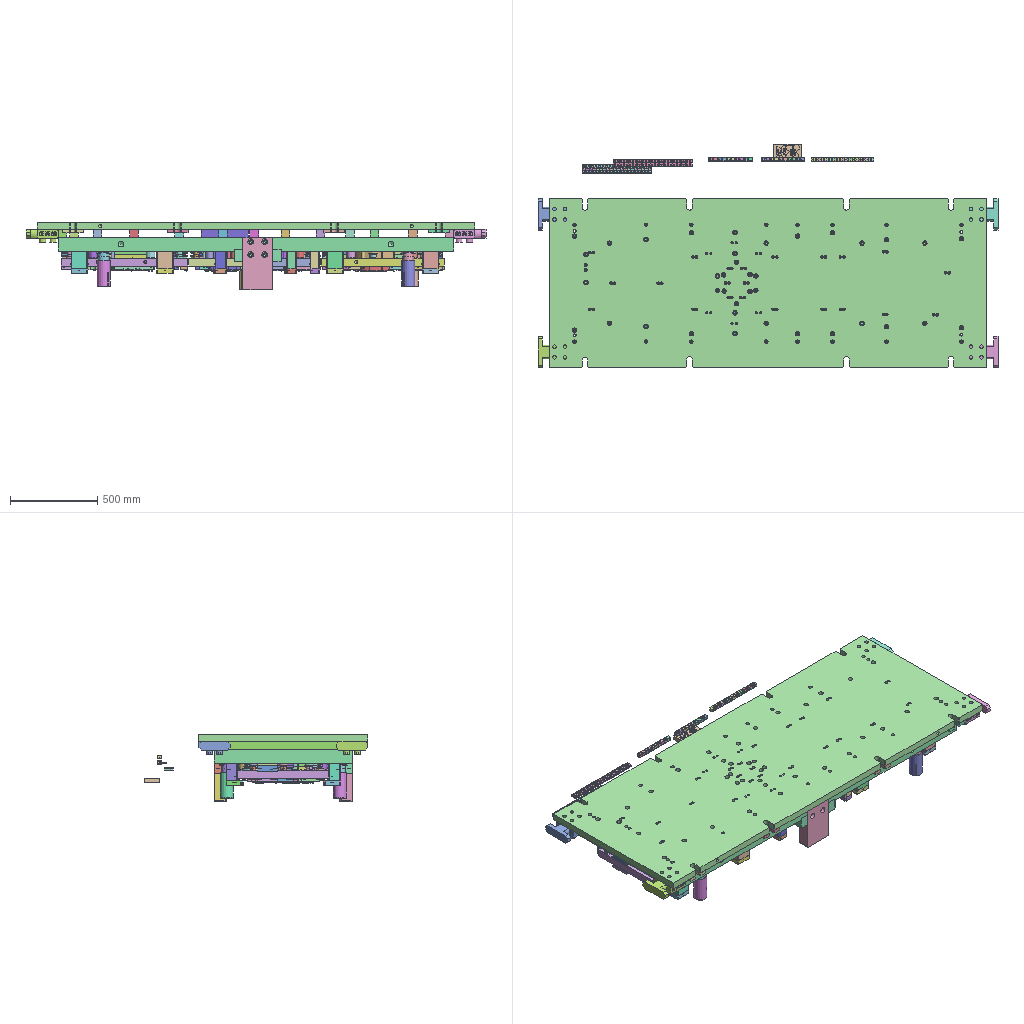Assembly | STEP file | 803 different items | 803 placed | box 2640 x 1282 x 385 mm
Parts list (item | name | quantity | parent item | size | volume), first 255 of 803 items:
1 | 1_id3214_x_t | x1 | in gslz 2016.10.28-10_x_t | 21 x 21 x 81 mm | 13603 mm3
2 | 1_id3210_x_t | x1 | in gslz 2016.10.28-10_x_t | 21 x 21 x 81 mm | 13603 mm3
3 | 1_id3206_x_t | x1 | in gslz 2016.10.28-10_x_t | 21 x 21 x 81 mm | 13603 mm3
4 | 1_id3202_x_t | x1 | in gslz 2016.10.28-10_x_t | 21 x 21 x 81 mm | 13603 mm3
5 | gslz 2016.10.28-10_id3198_x_t | x1 | in gslz 2016.10.28-10_x_t | 101.187 x 62.226 x 90 mm | 237811 mm3
6 | gslz 2016.10.28-10_id3194_x_t | x1 | in gslz 2016.10.28-10_x_t | 101.187 x 66.608 x 90 mm | 278822 mm3
7 | gslz 2016.10.28-10_id3190_x_t | x1 | in gslz 2016.10.28-10_x_t | 51.195 x 103.6 x 90 mm | 199398 mm3
8 | 107_id3186_x_t | x1 | in gslz 2016.10.28-10_x_t | 260 x 110 x 20 mm | 549192 mm3
9 | 105_id3182_x_t | x1 | in gslz 2016.10.28-10_x_t | 265 x 105 x 20 mm | 533692 mm3
10 | 106_id3178_x_t | x1 | in gslz 2016.10.28-10_x_t | 85 x 150 x 20 mm | 239795 mm3
11 | 108_id3174_x_t | x1 | in gslz 2016.10.28-10_x_t | 105 x 160 x 20 mm | 320795 mm3
12 | 109_id3170_x_t | x1 | in gslz 2016.10.28-10_x_t | 110 x 145 x 20 mm | 303795 mm3
13 | 406_id3166_x_t | x1 | in gslz 2016.10.28-10_x_t | 260 x 115 x 20 mm | 434950 mm3
14 | 408_id3162_x_t | x1 | in gslz 2016.10.28-10_x_t | 105 x 157 x 20 mm | 244863 mm3
15 | 409_id3158_x_t | x1 | in gslz 2016.10.28-10_x_t | 110 x 142 x 20 mm | 222515 mm3
16 | gslz 2016.10.28-10_id3154_x_t | x1 | in gslz 2016.10.28-10_x_t | 12.88 x 31.5 x 15.5 mm | 5788 mm3
17 | gslz 2016.10.28-10_id3150_x_t | x1 | in gslz 2016.10.28-10_x_t | 6 x 6 x 42 mm | 574.275 mm3
18 | gslz 2016.10.28-10_id3146_x_t | x1 | in gslz 2016.10.28-10_x_t | 6 x 6 x 42 mm | 574.275 mm3
19 | gslz 2016.10.28-10_id3142_x_t | x1 | in gslz 2016.10.28-10_x_t | 6 x 6 x 42 mm | 574.275 mm3
20 | gslz 2016.10.28-10_id3138_x_t | x1 | in gslz 2016.10.28-10_x_t | 6 x 6 x 40 mm | 848.23 mm3
21 | gslz 2016.10.28-10_id3134_x_t | x1 | in gslz 2016.10.28-10_x_t | 6 x 6 x 42 mm | 574.275 mm3
22 | gslz 2016.10.28-10_id3130_x_t | x1 | in gslz 2016.10.28-10_x_t | 6 x 6 x 40 mm | 848.23 mm3
23 | gslz 2016.10.28-10_id3126_x_t | x1 | in gslz 2016.10.28-10_x_t | 6 x 6 x 40 mm | 848.23 mm3
24 | gslz 2016.10.28-10_id3122_x_t | x1 | in gslz 2016.10.28-10_x_t | 6 x 6 x 40 mm | 848.23 mm3
25 | gslz 2016.10.28-10_id3118_x_t | x1 | in gslz 2016.10.28-10_x_t | 87.187 x 59.877 x 90 mm | 187380 mm3
26 | gslz 2016.10.28-10_id3114_x_t | x1 | in gslz 2016.10.28-10_x_t | 6 x 6 x 42 mm | 574.275 mm3
27 | gslz 2016.10.28-10_id3110_x_t | x1 | in gslz 2016.10.28-10_x_t | 6 x 6 x 40 mm | 848.23 mm3
28 | gslz 2016.10.28-10_id3106_x_t | x1 | in gslz 2016.10.28-10_x_t | 6 x 6 x 40 mm | 848.23 mm3
29 | gslz 2016.10.28-10_id3102_x_t | x1 | in gslz 2016.10.28-10_x_t | 6 x 6 x 42 mm | 574.275 mm3
30 | gslz 2016.10.28-10_id3098_x_t | x1 | in gslz 2016.10.28-10_x_t | 6 x 6 x 40 mm | 848.23 mm3
31 | gslz 2016.10.28-10_id3094_x_t | x1 | in gslz 2016.10.28-10_x_t | 6 x 6 x 42 mm | 574.275 mm3
32 | gslz 2016.10.28-10_id3090_x_t | x1 | in gslz 2016.10.28-10_x_t | 6 x 6 x 40 mm | 848.23 mm3
33 | gslz 2016.10.28-10_id3086_x_t | x1 | in gslz 2016.10.28-10_x_t | 6 x 6 x 42 mm | 574.275 mm3
34 | gslz 2016.10.28-10_id3082_x_t | x1 | in gslz 2016.10.28-10_x_t | 87.187 x 65.37 x 90 mm | 204585 mm3
35 | gslz 2016.10.28-10_id3078_x_t | x1 | in gslz 2016.10.28-10_x_t | 6 x 6 x 42 mm | 574.275 mm3
36 | gslz 2016.10.28-10_id3074_x_t | x1 | in gslz 2016.10.28-10_x_t | 6 x 6 x 42 mm | 574.275 mm3
37 | gslz 2016.10.28-10_id3070_x_t | x1 | in gslz 2016.10.28-10_x_t | 6 x 6 x 40 mm | 848.23 mm3
38 | gslz 2016.10.28-10_id3066_x_t | x1 | in gslz 2016.10.28-10_x_t | 6 x 6 x 40 mm | 848.23 mm3
39 | gslz 2016.10.28-10_id3062_x_t | x1 | in gslz 2016.10.28-10_x_t | 6 x 6 x 42 mm | 574.275 mm3
40 | gslz 2016.10.28-10_id3058_x_t | x1 | in gslz 2016.10.28-10_x_t | 6 x 6 x 40 mm | 848.23 mm3
41 | gslz 2016.10.28-10_id3054_x_t | x1 | in gslz 2016.10.28-10_x_t | 57.01 x 93.6 x 90 mm | 227783 mm3
42 | gslz 2016.10.28-10_id3050_x_t | x1 | in gslz 2016.10.28-10_x_t | 36.691 x 100 x 90 mm | 156614 mm3
43 | gslz 2016.10.28-10_id3046_x_t | x1 | in gslz 2016.10.28-10_x_t | 13 x 13 x 31 mm | 2308 mm3
44 | gslz 2016.10.28-10_id3042_x_t | x1 | in gslz 2016.10.28-10_x_t | 8 x 8 x 26 mm | 800.75 mm3
45 | gslz 2016.10.28-10_id3038_x_t | x1 | in gslz 2016.10.28-10_x_t | 8 x 8 x 26 mm | 800.75 mm3
46 | gslz 2016.10.28-10_id3034_x_t | x1 | in gslz 2016.10.28-10_x_t | 8 x 8 x 26 mm | 800.75 mm3
47 | gslz 2016.10.28-10_id3030_x_t | x1 | in gslz 2016.10.28-10_x_t | 13 x 13 x 31 mm | 2308 mm3
48 | gslz 2016.10.28-10_id3026_x_t | x1 | in gslz 2016.10.28-10_x_t | 8 x 8 x 26 mm | 800.75 mm3
49 | gslz 2016.10.28-10_id3022_x_t | x1 | in gslz 2016.10.28-10_x_t | 13 x 13 x 31 mm | 2308 mm3
50 | gslz 2016.10.28-10_id3018_x_t | x1 | in gslz 2016.10.28-10_x_t | 8 x 8 x 26 mm | 800.75 mm3
51 | gslz 2016.10.28-10_id3014_x_t | x1 | in gslz 2016.10.28-10_x_t | 8 x 8 x 26 mm | 800.75 mm3
52 | gslz 2016.10.28-10_id3010_x_t | x1 | in gslz 2016.10.28-10_x_t | 13 x 13 x 31 mm | 2308 mm3
53 | gslz 2016.10.28-10_id3006_x_t | x1 | in gslz 2016.10.28-10_x_t | 8 x 8 x 26 mm | 800.75 mm3
54 | gslz 2016.10.28-10_id3002_x_t | x1 | in gslz 2016.10.28-10_x_t | 8 x 8 x 26 mm | 800.75 mm3
55 | gslz 2016.10.28-10_id2998_x_t | x1 | in gslz 2016.10.28-10_x_t | 8 x 8 x 26 mm | 800.75 mm3
56 | gslz 2016.10.28-10_id2994_x_t | x1 | in gslz 2016.10.28-10_x_t | 13 x 13 x 31 mm | 2308 mm3
57 | 112_id2990_x_t | x1 | in gslz 2016.10.28-10_x_t | 185 x 135 x 20 mm | 472603 mm3
58 | gslz 2016.10.28-10_id2986_x_t | x1 | in gslz 2016.10.28-10_x_t | 134.015 x 80.135 x 90 mm | 527779 mm3
59 | gslz 2016.10.28-10_id2982_x_t | x1 | in gslz 2016.10.28-10_x_t | 6 x 6 x 42 mm | 574.275 mm3
60 | gslz 2016.10.28-10_id2978_x_t | x1 | in gslz 2016.10.28-10_x_t | 6 x 6 x 40 mm | 848.23 mm3
61 | gslz 2016.10.28-10_id2974_x_t | x1 | in gslz 2016.10.28-10_x_t | 6 x 6 x 42 mm | 574.275 mm3
62 | gslz 2016.10.28-10_id2970_x_t | x1 | in gslz 2016.10.28-10_x_t | 6 x 6 x 40 mm | 848.23 mm3
63 | 111_id2966_x_t | x1 | in gslz 2016.10.28-10_x_t | 180 x 95 x 20 mm | 326795 mm3
64 | gslz 2016.10.28-10_id2962_x_t | x1 | in gslz 2016.10.28-10_x_t | 6 x 6 x 40 mm | 848.23 mm3
65 | gslz 2016.10.28-10_id2958_x_t | x1 | in gslz 2016.10.28-10_x_t | 6 x 6 x 42 mm | 574.275 mm3
66 | gslz 2016.10.28-10_id2954_x_t | x1 | in gslz 2016.10.28-10_x_t | 6 x 6 x 42 mm | 574.275 mm3
67 | gslz 2016.10.28-10_id2950_x_t | x1 | in gslz 2016.10.28-10_x_t | 6 x 6 x 40 mm | 848.23 mm3
68 | gslz 2016.10.28-10_id2946_x_t | x1 | in gslz 2016.10.28-10_x_t | 129.443 x 37.474 x 90 mm | 310631 mm3
69 | gslz 2016.10.28-10_id2942_x_t | x1 | in gslz 2016.10.28-10_x_t | 6 x 6 x 42 mm | 574.275 mm3
70 | gslz 2016.10.28-10_id2938_x_t | x1 | in gslz 2016.10.28-10_x_t | 6 x 6 x 40 mm | 848.23 mm3
71 | gslz 2016.10.28-10_id2934_x_t | x1 | in gslz 2016.10.28-10_x_t | 6 x 6 x 42 mm | 574.275 mm3
72 | gslz 2016.10.28-10_id2930_x_t | x1 | in gslz 2016.10.28-10_x_t | 6 x 6 x 40 mm | 848.23 mm3
73 | gslz 2016.10.28-10_id2926_x_t | x1 | in gslz 2016.10.28-10_x_t | 6 x 6 x 42 mm | 574.275 mm3
74 | gslz 2016.10.28-10_id2922_x_t | x1 | in gslz 2016.10.28-10_x_t | 6 x 6 x 40 mm | 848.23 mm3
75 | gslz 2016.10.28-10_id2918_x_t | x1 | in gslz 2016.10.28-10_x_t | 6 x 6 x 40 mm | 848.23 mm3
76 | gslz 2016.10.28-10_id2914_x_t | x1 | in gslz 2016.10.28-10_x_t | 6 x 6 x 42 mm | 574.275 mm3
77 | 110_id2910_x_t | x1 | in gslz 2016.10.28-10_x_t | 195 x 140 x 20 mm | 526993 mm3
78 | gslz 2016.10.28-10_id2906_x_t | x1 | in gslz 2016.10.28-10_x_t | 54.788 x 54 x 90 mm | 215113 mm3
79 | gslz 2016.10.28-10_id2902_x_t | x1 | in gslz 2016.10.28-10_x_t | 64.28 x 75.342 x 90 mm | 328224 mm3
80 | 1_id2898_x_t | x1 | in gslz 2016.10.28-10_x_t | 15 x 15 x 91 mm | 7738 mm3
81 | gslz 2016.10.28-10_id2894_x_t | x1 | in gslz 2016.10.28-10_x_t | 30.933 x 36.163 x 93 mm | 43152 mm3
82 | gslz 2016.10.28-10_id2890_x_t | x1 | in gslz 2016.10.28-10_x_t | 62 x 25 x 90 mm | 116529 mm3
83 | gslz 2016.10.28-10_id2886_x_t | x1 | in gslz 2016.10.28-10_x_t | 32.472 x 35.825 x 93 mm | 45038 mm3
84 | gslz 2016.10.28-10_id2882_x_t | x1 | in gslz 2016.10.28-10_x_t | 34.187 x 36.414 x 93 mm | 46333 mm3
85 | gslz 2016.10.28-10_id2878_x_t | x1 | in gslz 2016.10.28-10_x_t | 148.369 x 39.226 x 90 mm | 378722 mm3
86 | gslz 2016.10.28-10_id2874_x_t | x1 | in gslz 2016.10.28-10_x_t | 30.689 x 35.785 x 93 mm | 42819 mm3
87 | gslz 2016.10.28-10_id2870_x_t | x1 | in gslz 2016.10.28-10_x_t | 60 x 27 x 90 mm | 122829 mm3
88 | 1_id2866_x_t | x1 | in gslz 2016.10.28-10_x_t | 18 x 18 x 91 mm | 11747 mm3
89 | 1_id2862_x_t | x1 | in gslz 2016.10.28-10_x_t | 18 x 18 x 91 mm | 11747 mm3
90 | 1_id2858_x_t | x1 | in gslz 2016.10.28-10_x_t | 15 x 15 x 91 mm | 7738 mm3
91 | 117_id2854_x_t | x1 | in gslz 2016.10.28-10_x_t | 115 x 80 x 20 mm | 163028 mm3
92 | 115_id2850_x_t | x1 | in gslz 2016.10.28-10_x_t | 109 x 70 x 20 mm | 139295 mm3
93 | gslz 2016.10.28-10_id2846_x_t | x1 | in gslz 2016.10.28-10_x_t | 6 x 6 x 40 mm | 848.23 mm3
94 | gslz 2016.10.28-10_id2842_x_t | x1 | in gslz 2016.10.28-10_x_t | 6 x 6 x 42 mm | 574.275 mm3
95 | gslz 2016.10.28-10_id2838_x_t | x1 | in gslz 2016.10.28-10_x_t | 6 x 6 x 42 mm | 574.275 mm3
96 | gslz 2016.10.28-10_id2834_x_t | x1 | in gslz 2016.10.28-10_x_t | 6 x 6 x 40 mm | 848.23 mm3
97 | gslz 2016.10.28-10_id2830_x_t | x1 | in gslz 2016.10.28-10_x_t | 6 x 6 x 42 mm | 574.275 mm3
98 | gslz 2016.10.28-10_id2826_x_t | x1 | in gslz 2016.10.28-10_x_t | 6 x 6 x 40 mm | 848.23 mm3
99 | gslz 2016.10.28-10_id2822_x_t | x1 | in gslz 2016.10.28-10_x_t | 6 x 6 x 42 mm | 574.275 mm3
100 | gslz 2016.10.28-10_id2818_x_t | x1 | in gslz 2016.10.28-10_x_t | 6 x 6 x 40 mm | 848.23 mm3
101 | gslz 2016.10.28-10_id2814_x_t | x1 | in gslz 2016.10.28-10_x_t | 6 x 6 x 40 mm | 848.23 mm3
102 | gslz 2016.10.28-10_id2810_x_t | x1 | in gslz 2016.10.28-10_x_t | 6 x 6 x 42 mm | 574.275 mm3
103 | gslz 2016.10.28-10_id2806_x_t | x1 | in gslz 2016.10.28-10_x_t | 6 x 6 x 42 mm | 574.275 mm3
104 | gslz 2016.10.28-10_id2802_x_t | x1 | in gslz 2016.10.28-10_x_t | 6 x 6 x 40 mm | 848.23 mm3
105 | gslz 2016.10.28-10_id2798_x_t | x1 | in gslz 2016.10.28-10_x_t | 139.573 x 57.5 x 90 mm | 377716 mm3
106 | 419_id2794_x_t | x1 | in gslz 2016.10.28-10_x_t | 195 x 140 x 21.724 mm | 388406 mm3
107 | 429_id2790_x_t | x1 | in gslz 2016.10.28-10_x_t | 135 x 70 x 20 mm | 140686 mm3
108 | 430_id2786_x_t | x1 | in gslz 2016.10.28-10_x_t | 165 x 80 x 20 mm | 194228 mm3
109 | 113_id2782_x_t | x1 | in gslz 2016.10.28-10_x_t | 125 x 75 x 20 mm | 174195 mm3
110 | 116_id2778_x_t | x1 | in gslz 2016.10.28-10_x_t | 130 x 85 x 20 mm | 205795 mm3
111 | gslz 2016.10.28-10_id2774_x_t | x1 | in gslz 2016.10.28-10_x_t | 8 x 8 x 26 mm | 800.75 mm3
112 | gslz 2016.10.28-10_id2770_x_t | x1 | in gslz 2016.10.28-10_x_t | 8 x 8 x 26 mm | 800.75 mm3
113 | gslz 2016.10.28-10_id2766_x_t | x1 | in gslz 2016.10.28-10_x_t | 13 x 13 x 31 mm | 2308 mm3
114 | gslz 2016.10.28-10_id2762_x_t | x1 | in gslz 2016.10.28-10_x_t | 8 x 8 x 26 mm | 800.75 mm3
115 | gslz 2016.10.28-10_id2758_x_t | x1 | in gslz 2016.10.28-10_x_t | 13 x 13 x 31 mm | 2308 mm3
116 | gslz 2016.10.28-10_id2754_x_t | x1 | in gslz 2016.10.28-10_x_t | 8 x 8 x 26 mm | 800.75 mm3
117 | gslz 2016.10.28-10_id2750_x_t | x1 | in gslz 2016.10.28-10_x_t | 13 x 13 x 31 mm | 2308 mm3
118 | gslz 2016.10.28-10_id2746_x_t | x1 | in gslz 2016.10.28-10_x_t | 13 x 13 x 31 mm | 2308 mm3
119 | gslz 2016.10.28-10_id2742_x_t | x1 | in gslz 2016.10.28-10_x_t | 13 x 13 x 31 mm | 2308 mm3
120 | gslz 2016.10.28-10_id2738_x_t | x1 | in gslz 2016.10.28-10_x_t | 13 x 13 x 31 mm | 2308 mm3
121 | gslz 2016.10.28-10_id2734_x_t | x1 | in gslz 2016.10.28-10_x_t | 8 x 8 x 26 mm | 800.75 mm3
122 | gslz 2016.10.28-10_id2730_x_t | x1 | in gslz 2016.10.28-10_x_t | 8 x 8 x 26 mm | 800.75 mm3
123 | gslz 2016.10.28-10_id2726_x_t | x1 | in gslz 2016.10.28-10_x_t | 8 x 8 x 26 mm | 800.75 mm3
124 | 407_id2722_x_t | x1 | in gslz 2016.10.28-10_x_t | 70 x 140 x 20 mm | 171561 mm3
125 | gslz 2016.10.28-10_id2718_x_t | x1 | in gslz 2016.10.28-10_x_t | 8 x 8 x 26 mm | 800.75 mm3
126 | gslz 2016.10.28-10_id2714_x_t | x1 | in gslz 2016.10.28-10_x_t | 13 x 13 x 31 mm | 2308 mm3
127 | gslz 2016.10.28-10_id2710_x_t | x1 | in gslz 2016.10.28-10_x_t | 13 x 13 x 31 mm | 2308 mm3
128 | gslz 2016.10.28-10_id2706_x_t | x1 | in gslz 2016.10.28-10_x_t | 8 x 8 x 18 mm | 574.556 mm3
129 | gslz 2016.10.28-10_id2702_x_t | x1 | in gslz 2016.10.28-10_x_t | 8 x 8 x 18 mm | 574.556 mm3
130 | gslz 2016.10.28-10_id2698_x_t | x1 | in gslz 2016.10.28-10_x_t | 8 x 8 x 15 mm | 565.487 mm3
131 | gslz 2016.10.28-10_id2694_x_t | x1 | in gslz 2016.10.28-10_x_t | 8 x 8 x 15 mm | 565.487 mm3
132 | gslz 2016.10.28-10_id2690_x_t | x1 | in gslz 2016.10.28-10_x_t | 8 x 8 x 15 mm | 565.487 mm3
133 | gslz 2016.10.28-10_id2686_x_t | x1 | in gslz 2016.10.28-10_x_t | 8 x 8 x 18 mm | 574.556 mm3
134 | gslz 2016.10.28-10_id2682_x_t | x1 | in gslz 2016.10.28-10_x_t | 8 x 8 x 18 mm | 574.556 mm3
135 | gslz 2016.10.28-10_id2678_x_t | x1 | in gslz 2016.10.28-10_x_t | 8 x 8 x 15 mm | 565.487 mm3
136 | gslz 2016.10.28-10_id2674_x_t | x1 | in gslz 2016.10.28-10_x_t | 13 x 13 x 31 mm | 2308 mm3
137 | gslz 2016.10.28-10_id2670_x_t | x1 | in gslz 2016.10.28-10_x_t | 13 x 13 x 31 mm | 2308 mm3
138 | gslz 2016.10.28-10_id2666_x_t | x1 | in gslz 2016.10.28-10_x_t | 8 x 8 x 26 mm | 800.75 mm3
139 | gslz 2016.10.28-10_id2662_x_t | x1 | in gslz 2016.10.28-10_x_t | 8 x 8 x 26 mm | 800.75 mm3
140 | gslz 2016.10.28-10_id2658_x_t | x1 | in gslz 2016.10.28-10_x_t | 8 x 8 x 26 mm | 800.75 mm3
141 | gslz 2016.10.28-10_id2654_x_t | x1 | in gslz 2016.10.28-10_x_t | 8 x 8 x 26 mm | 800.75 mm3
142 | gslz 2016.10.28-10_id2650_x_t | x1 | in gslz 2016.10.28-10_x_t | 13 x 13 x 31 mm | 2308 mm3
143 | gslz 2016.10.28-10_id2646_x_t | x1 | in gslz 2016.10.28-10_x_t | 13 x 13 x 31 mm | 2308 mm3
144 | gslz 2016.10.28-10_id2642_x_t | x1 | in gslz 2016.10.28-10_x_t | 8 x 8 x 26 mm | 800.75 mm3
145 | gslz 2016.10.28-10_id2638_x_t | x1 | in gslz 2016.10.28-10_x_t | 8 x 8 x 26 mm | 800.75 mm3
146 | gslz 2016.10.28-10_id2634_x_t | x1 | in gslz 2016.10.28-10_x_t | 8 x 8 x 26 mm | 800.75 mm3
147 | gslz 2016.10.28-10_id2630_x_t | x1 | in gslz 2016.10.28-10_x_t | 8 x 8 x 26 mm | 800.75 mm3
148 | gslz 2016.10.28-10_id2626_x_t | x1 | in gslz 2016.10.28-10_x_t | 13 x 13 x 31 mm | 2308 mm3
149 | gslz 2016.10.28-10_id2622_x_t | x1 | in gslz 2016.10.28-10_x_t | 13 x 13 x 31 mm | 2308 mm3
150 | gslz 2016.10.28-10_id2618_x_t | x1 | in gslz 2016.10.28-10_x_t | 8 x 8 x 26 mm | 800.75 mm3
151 | gslz 2016.10.28-10_id2614_x_t | x1 | in gslz 2016.10.28-10_x_t | 8 x 8 x 26 mm | 800.75 mm3
152 | gslz 2016.10.28-10_id2610_x_t | x1 | in gslz 2016.10.28-10_x_t | 8 x 8 x 26 mm | 800.75 mm3
153 | gslz 2016.10.28-10_id2606_x_t | x1 | in gslz 2016.10.28-10_x_t | 8 x 8 x 26 mm | 800.75 mm3
154 | gslz 2016.10.28-10_id2602_x_t | x1 | in gslz 2016.10.28-10_x_t | 4 x 4 x 42 mm | 159.922 mm3
155 | gslz 2016.10.28-10_id2598_x_t | x1 | in gslz 2016.10.28-10_x_t | 4 x 4 x 42 mm | 159.922 mm3
156 | gslz 2016.10.28-10_id2594_x_t | x1 | in gslz 2016.10.28-10_x_t | 4 x 4 x 42 mm | 159.924 mm3
157 | gslz 2016.10.28-10_id2590_x_t | x1 | in gslz 2016.10.28-10_x_t | 4 x 4 x 42 mm | 159.924 mm3
158 | 426_id2586_x_t | x1 | in gslz 2016.10.28-10_x_t | 70 x 50 x 20 mm | 56753 mm3
159 | gslz 2016.10.28-10_id2582_x_t | x1 | in gslz 2016.10.28-10_x_t | 8 x 8 x 26 mm | 800.75 mm3
160 | gslz 2016.10.28-10_id2578_x_t | x1 | in gslz 2016.10.28-10_x_t | 13 x 13 x 31 mm | 2308 mm3
161 | gslz 2016.10.28-10_id2574_x_t | x1 | in gslz 2016.10.28-10_x_t | 13 x 13 x 31 mm | 2308 mm3
162 | gslz 2016.10.28-10_id2570_x_t | x1 | in gslz 2016.10.28-10_x_t | 8 x 8 x 26 mm | 800.75 mm3
163 | gslz 2016.10.28-10_id2566_x_t | x1 | in gslz 2016.10.28-10_x_t | 8 x 8 x 26 mm | 800.75 mm3
164 | gslz 2016.10.28-10_id2562_x_t | x1 | in gslz 2016.10.28-10_x_t | 8 x 8 x 26 mm | 800.75 mm3
165 | gslz 2016.10.28-10_id2558_x_t | x1 | in gslz 2016.10.28-10_x_t | 8 x 8 x 26 mm | 800.75 mm3
166 | gslz 2016.10.28-10_id2554_x_t | x1 | in gslz 2016.10.28-10_x_t | 13 x 13 x 31 mm | 2308 mm3
167 | gslz 2016.10.28-10_id2550_x_t | x1 | in gslz 2016.10.28-10_x_t | 13 x 13 x 31 mm | 2308 mm3
168 | gslz 2016.10.28-10_id2546_x_t | x1 | in gslz 2016.10.28-10_x_t | 8 x 8 x 26 mm | 800.75 mm3
169 | gslz 2016.10.28-10_id2542_x_t | x1 | in gslz 2016.10.28-10_x_t | 8 x 8 x 26 mm | 800.75 mm3
170 | gslz 2016.10.28-10_id2538_x_t | x1 | in gslz 2016.10.28-10_x_t | 8 x 8 x 26 mm | 800.75 mm3
171 | gslz 2016.10.28-10_id2534_x_t | x1 | in gslz 2016.10.28-10_x_t | 8 x 8 x 26 mm | 800.75 mm3
172 | gslz 2016.10.28-10_id2530_x_t | x1 | in gslz 2016.10.28-10_x_t | 13 x 13 x 31 mm | 2308 mm3
173 | gslz 2016.10.28-10_id2526_x_t | x1 | in gslz 2016.10.28-10_x_t | 13 x 13 x 31 mm | 2308 mm3
174 | gslz 2016.10.28-10_id2522_x_t | x1 | in gslz 2016.10.28-10_x_t | 8 x 8 x 26 mm | 800.75 mm3
175 | gslz 2016.10.28-10_id2518_x_t | x1 | in gslz 2016.10.28-10_x_t | 8 x 8 x 26 mm | 800.75 mm3
176 | gslz 2016.10.28-10_id2514_x_t | x1 | in gslz 2016.10.28-10_x_t | 8 x 8 x 26 mm | 800.75 mm3
177 | gslz 2016.10.28-10_id2510_x_t | x1 | in gslz 2016.10.28-10_x_t | 8 x 8 x 26 mm | 800.75 mm3
178 | gslz 2016.10.28-10_id2506_x_t | x1 | in gslz 2016.10.28-10_x_t | 13 x 13 x 31 mm | 2308 mm3
179 | gslz 2016.10.28-10_id2502_x_t | x1 | in gslz 2016.10.28-10_x_t | 13 x 13 x 31 mm | 2308 mm3
180 | gslz 2016.10.28-10_id2498_x_t | x1 | in gslz 2016.10.28-10_x_t | 8 x 8 x 26 mm | 800.75 mm3
181 | gslz 2016.10.28-10_id2494_x_t | x1 | in gslz 2016.10.28-10_x_t | 8 x 8 x 26 mm | 800.75 mm3
182 | 424_id2490_x_t | x1 | in gslz 2016.10.28-10_x_t | 70 x 50 x 20 mm | 59956 mm3
183 | 420_id2486_x_t | x1 | in gslz 2016.10.28-10_x_t | 50 x 60 x 20 mm | 47706 mm3
184 | 425_id2482_x_t | x1 | in gslz 2016.10.28-10_x_t | 70 x 50 x 20 mm | 59956 mm3
185 | gslz 2016.10.28-10_id2478_x_t | x1 | in gslz 2016.10.28-10_x_t | 8 x 8 x 26 mm | 800.75 mm3
186 | 421_id2474_x_t | x1 | in gslz 2016.10.28-10_x_t | 50 x 60 x 20 mm | 49706 mm3
187 | gslz 2016.10.28-10_id2470_x_t | x1 | in gslz 2016.10.28-10_x_t | 8 x 8 x 26 mm | 800.75 mm3
188 | gslz 2016.10.28-10_id2466_x_t | x1 | in gslz 2016.10.28-10_x_t | 6 x 6 x 40 mm | 848.23 mm3
189 | gslz 2016.10.28-10_id2462_x_t | x1 | in gslz 2016.10.28-10_x_t | 6 x 6 x 42 mm | 574.275 mm3
190 | gslz 2016.10.28-10_id2458_x_t | x1 | in gslz 2016.10.28-10_x_t | 50 x 50 x 40 mm | 71266 mm3
191 | gslz 2016.10.28-10_id2454_x_t | x1 | in gslz 2016.10.28-10_x_t | 50 x 50 x 40 mm | 71266 mm3
192 | gslz 2016.10.28-10_id2450_x_t | x1 | in gslz 2016.10.28-10_x_t | 50 x 50 x 40 mm | 71266 mm3
193 | gslz 2016.10.28-10_id2446_x_t | x1 | in gslz 2016.10.28-10_x_t | 50 x 50 x 40 mm | 71266 mm3
194 | gslz 2016.10.28-10_id2442_x_t | x1 | in gslz 2016.10.28-10_x_t | 40 x 40 x 40 mm | 45553 mm3
195 | gslz 2016.10.28-10_id2438_x_t | x1 | in gslz 2016.10.28-10_x_t | 50 x 50 x 40 mm | 71266 mm3
196 | gslz 2016.10.28-10_id2434_x_t | x1 | in gslz 2016.10.28-10_x_t | 50 x 50 x 40 mm | 71266 mm3
197 | gslz 2016.10.28-10_id2430_x_t | x1 | in gslz 2016.10.28-10_x_t | 50 x 50 x 40 mm | 71266 mm3
198 | gslz 2016.10.28-10_id2426_x_t | x1 | in gslz 2016.10.28-10_x_t | 50 x 50 x 40 mm | 71266 mm3
199 | gslz 2016.10.28-10_id2422_x_t | x1 | in gslz 2016.10.28-10_x_t | 95 x 20 x 15 mm | 25916 mm3
200 | gslz 2016.10.28-10_id2418_x_t | x1 | in gslz 2016.10.28-10_x_t | 8 x 8 x 26 mm | 800.75 mm3
201 | gslz 2016.10.28-10_id2414_x_t | x1 | in gslz 2016.10.28-10_x_t | 8 x 8 x 26 mm | 800.75 mm3
202 | gslz 2016.10.28-10_id2410_x_t | x1 | in gslz 2016.10.28-10_x_t | 13 x 13 x 31 mm | 2308 mm3
203 | gslz 2016.10.28-10_id2406_x_t | x1 | in gslz 2016.10.28-10_x_t | 8 x 8 x 26 mm | 800.75 mm3
204 | 413_id2402_x_t | x1 | in gslz 2016.10.28-10_x_t | 55 x 52 x 20 mm | 45753 mm3
205 | gslz 2016.10.28-10_id2398_x_t | x1 | in gslz 2016.10.28-10_x_t | 8 x 8 x 26 mm | 800.75 mm3
206 | 411_id2394_x_t | x1 | in gslz 2016.10.28-10_x_t | 55 x 52 x 20 mm | 46099 mm3
207 | gslz 2016.10.28-10_id2390_x_t | x1 | in gslz 2016.10.28-10_x_t | 8 x 8 x 26 mm | 800.75 mm3
208 | gslz 2016.10.28-10_id2386_x_t | x1 | in gslz 2016.10.28-10_x_t | 8 x 8 x 26 mm | 800.75 mm3
209 | gslz 2016.10.28-10_id2382_x_t | x1 | in gslz 2016.10.28-10_x_t | 13 x 13 x 31 mm | 2308 mm3
210 | gslz 2016.10.28-10_id2378_x_t | x1 | in gslz 2016.10.28-10_x_t | 8 x 8 x 26 mm | 800.75 mm3
211 | 1_id2374_x_t | x1 | in gslz 2016.10.28-10_x_t | 40 x 40 x 20 mm | 20116 mm3
212 | 1_id2370_x_t | x1 | in gslz 2016.10.28-10_x_t | 40 x 40 x 20 mm | 20116 mm3
213 | 1_id2366_x_t | x1 | in gslz 2016.10.28-10_x_t | 40 x 40 x 20 mm | 20116 mm3
214 | 1_id2362_x_t | x1 | in gslz 2016.10.28-10_x_t | 24 x 24 x 100 mm | 18465 mm3
215 | 1_id2358_x_t | x1 | in gslz 2016.10.28-10_x_t | 24 x 24 x 100 mm | 18465 mm3
216 | 1_id2354_x_t | x1 | in gslz 2016.10.28-10_x_t | 24 x 24 x 100 mm | 18465 mm3
217 | 1_id2350_x_t | x1 | in gslz 2016.10.28-10_x_t | 24 x 24 x 100 mm | 18465 mm3
218 | gslz 2016.10.28-10_id2346_x_t | x1 | in gslz 2016.10.28-10_x_t | 45 x 25 x 60 mm | 46550 mm3
219 | gslz 2016.10.28-10_id2342_x_t | x1 | in gslz 2016.10.28-10_x_t | 43 x 23 x 60 mm | 38390 mm3
220 | gslz 2016.10.28-10_id2338_x_t | x1 | in gslz 2016.10.28-10_x_t | 38 x 21 x 60 mm | 33724 mm3
221 | 114_id2334_x_t | x1 | in gslz 2016.10.28-10_x_t | 200 x 245 x 20 mm | 862921 mm3
222 | gslz 2016.10.28-10_id2330_x_t | x1 | in gslz 2016.10.28-10_x_t | 25 x 60 x 27.5 mm | 33698 mm3
223 | 302_id2326_x_t | x1 | in gslz 2016.10.28-10_x_t | 370 x 122 x 45 mm | 1312955 mm3
224 | 301_id2322_x_t | x1 | in gslz 2016.10.28-10_x_t | 370 x 122 x 45 mm | 1311986 mm3
225 | gslz 2016.10.28-10_id2318_x_t | x1 | in gslz 2016.10.28-10_x_t | 95 x 20 x 15 mm | 25916 mm3
226 | gslz 2016.10.28-10_id2314_x_t | x1 | in gslz 2016.10.28-10_x_t | 65 x 20 x 10 mm | 11366 mm3
227 | gslz 2016.10.28-10_id2310_x_t | x1 | in gslz 2016.10.28-10_x_t | 95 x 20 x 15 mm | 25916 mm3
228 | gslz 2016.10.28-10_id2306_x_t | x1 | in gslz 2016.10.28-10_x_t | 95 x 20 x 15 mm | 25916 mm3
229 | 1_id2302_x_t | x1 | in gslz 2016.10.28-10_x_t | 40 x 40 x 20 mm | 20116 mm3
230 | 1_id2298_x_t | x1 | in gslz 2016.10.28-10_x_t | 24 x 24 x 100 mm | 18465 mm3
231 | 1_id2294_x_t | x1 | in gslz 2016.10.28-10_x_t | 24 x 24 x 100 mm | 18465 mm3
232 | 400_id2290_x_t | x1 | in gslz 2016.10.28-10_x_t | 140 x 110 x 20 mm | 176767 mm3
233 | gslz 2016.10.28-10_id2286_x_t | x1 | in gslz 2016.10.28-10_x_t | 50 x 50 x 40 mm | 71266 mm3
234 | gslz 2016.10.28-10_id2282_x_t | x1 | in gslz 2016.10.28-10_x_t | 50 x 50 x 40 mm | 71266 mm3
235 | gslz 2016.10.28-10_id2278_x_t | x1 | in gslz 2016.10.28-10_x_t | 50 x 50 x 40 mm | 71266 mm3
236 | gslz 2016.10.28-10_id2274_x_t | x1 | in gslz 2016.10.28-10_x_t | 50 x 50 x 40 mm | 70960 mm3
237 | 405_id2270_x_t | x1 | in gslz 2016.10.28-10_x_t | 85 x 150 x 20 mm | 196124 mm3
238 | gslz 2016.10.28-10_id2266_x_t | x1 | in gslz 2016.10.28-10_x_t | 80 x 74 x 90 mm | 484715 mm3
239 | 210_id2262_x_t | x1 | in gslz 2016.10.28-10_x_t | 220 x 305 x 70 mm | 3957216 mm3
240 | gslz 2016.10.28-10_id2258_x_t | x1 | in gslz 2016.10.28-10_x_t | 120 x 85 x 20 mm | 154255 mm3
241 | 001_id2254_x_t | x1 | in gslz 2016.10.28-10_x_t | 2510 x 970 x 40 mm | 95269879 mm3
242 | gslz 2016.10.28-10_id2250_x_t | x1 | in gslz 2016.10.28-10_x_t | 120 x 85 x 20 mm | 154255 mm3
243 | 027_id2246_x_t | x1 | in gslz 2016.10.28-10_x_t | 120 x 85 x 20 mm | 154255 mm3
244 | gslz 2016.10.28-10_id2242_x_t | x1 | in gslz 2016.10.28-10_x_t | 120 x 85 x 20 mm | 157455 mm3
245 | gslz 2016.10.28-10_id2238_x_t | x1 | in gslz 2016.10.28-10_x_t | 120 x 85 x 20 mm | 154255 mm3
246 | gslz 2016.10.28-10_id2234_x_t | x1 | in gslz 2016.10.28-10_x_t | 120 x 85 x 20 mm | 154255 mm3
247 | gslz 2016.10.28-10_id2230_x_t | x1 | in gslz 2016.10.28-10_x_t | 120 x 85 x 20 mm | 154255 mm3
248 | gslz 2016.10.28-10_id2226_x_t | x1 | in gslz 2016.10.28-10_x_t | 120 x 85 x 20 mm | 154255 mm3
249 | 011_id2222_x_t | x1 | in gslz 2016.10.28-10_x_t | 50 x 790 x 45 mm | 1720407 mm3
250 | 026_id2218_x_t | x1 | in gslz 2016.10.28-10_x_t | 50 x 790 x 45 mm | 1720407 mm3
251 | 015_id2214_x_t | x1 | in gslz 2016.10.28-10_x_t | 50 x 790 x 45 mm | 1647676 mm3
252 | 021_id2210_x_t | x1 | in gslz 2016.10.28-10_x_t | 50 x 790 x 45 mm | 1744458 mm3
253 | 022_id2206_x_t | x1 | in gslz 2016.10.28-10_x_t | 50 x 790 x 45 mm | 1744458 mm3
254 | 024_id2202_x_t | x1 | in gslz 2016.10.28-10_x_t | 50 x 790 x 45 mm | 1716749 mm3
255 | 014_id2198_x_t | x1 | in gslz 2016.10.28-10_x_t | 50 x 790 x 45 mm | 1744458 mm3
Placements (level | parent | child | x y z in mm | rotation matrix by rows), first 181 of 803 lines:
1 | gslz 2016.10.28-10_x_t | 1_id3214_x_t | 0.0 0.0 0.0 | 1 0 0 0 1 0 0 0 1
1 | gslz 2016.10.28-10_x_t | 1_id3210_x_t | 0.0 0.0 0.0 | 1 0 0 0 1 0 0 0 1
1 | gslz 2016.10.28-10_x_t | 1_id3206_x_t | 0.0 0.0 0.0 | 1 0 0 0 1 0 0 0 1
1 | gslz 2016.10.28-10_x_t | 1_id3202_x_t | 0.0 0.0 0.0 | 1 0 0 0 1 0 0 0 1
1 | gslz 2016.10.28-10_x_t | gslz 2016.10.28-10_id3198_x_t | 0.0 0.0 0.0 | 1 0 0 0 1 0 0 0 1
1 | gslz 2016.10.28-10_x_t | gslz 2016.10.28-10_id3194_x_t | 0.0 0.0 0.0 | 1 0 0 0 1 0 0 0 1
1 | gslz 2016.10.28-10_x_t | gslz 2016.10.28-10_id3190_x_t | 0.0 0.0 0.0 | 1 0 0 0 1 0 0 0 1
1 | gslz 2016.10.28-10_x_t | 107_id3186_x_t | 0.0 0.0 0.0 | 1 0 0 0 1 0 0 0 1
1 | gslz 2016.10.28-10_x_t | 105_id3182_x_t | 0.0 0.0 0.0 | 1 0 0 0 1 0 0 0 1
1 | gslz 2016.10.28-10_x_t | 106_id3178_x_t | 0.0 0.0 0.0 | 1 0 0 0 1 0 0 0 1
1 | gslz 2016.10.28-10_x_t | 108_id3174_x_t | 0.0 0.0 0.0 | 1 0 0 0 1 0 0 0 1
1 | gslz 2016.10.28-10_x_t | 109_id3170_x_t | 0.0 0.0 0.0 | 1 0 0 0 1 0 0 0 1
1 | gslz 2016.10.28-10_x_t | 406_id3166_x_t | 0.0 0.0 0.0 | 1 0 0 0 1 0 0 0 1
1 | gslz 2016.10.28-10_x_t | 408_id3162_x_t | 0.0 0.0 0.0 | 1 0 0 0 1 0 0 0 1
1 | gslz 2016.10.28-10_x_t | 409_id3158_x_t | 0.0 0.0 0.0 | 1 0 0 0 1 0 0 0 1
1 | gslz 2016.10.28-10_x_t | gslz 2016.10.28-10_id3154_x_t | 0.0 0.0 0.0 | 1 0 0 0 1 0 0 0 1
1 | gslz 2016.10.28-10_x_t | gslz 2016.10.28-10_id3150_x_t | 0.0 0.0 0.0 | 1 0 0 0 1 0 0 0 1
1 | gslz 2016.10.28-10_x_t | gslz 2016.10.28-10_id3146_x_t | 0.0 0.0 0.0 | 1 0 0 0 1 0 0 0 1
1 | gslz 2016.10.28-10_x_t | gslz 2016.10.28-10_id3142_x_t | 0.0 0.0 0.0 | 1 0 0 0 1 0 0 0 1
1 | gslz 2016.10.28-10_x_t | gslz 2016.10.28-10_id3138_x_t | 0.0 0.0 0.0 | 1 0 0 0 1 0 0 0 1
1 | gslz 2016.10.28-10_x_t | gslz 2016.10.28-10_id3134_x_t | 0.0 0.0 0.0 | 1 0 0 0 1 0 0 0 1
1 | gslz 2016.10.28-10_x_t | gslz 2016.10.28-10_id3130_x_t | 0.0 0.0 0.0 | 1 0 0 0 1 0 0 0 1
1 | gslz 2016.10.28-10_x_t | gslz 2016.10.28-10_id3126_x_t | 0.0 0.0 0.0 | 1 0 0 0 1 0 0 0 1
1 | gslz 2016.10.28-10_x_t | gslz 2016.10.28-10_id3122_x_t | 0.0 0.0 0.0 | 1 0 0 0 1 0 0 0 1
1 | gslz 2016.10.28-10_x_t | gslz 2016.10.28-10_id3118_x_t | 0.0 0.0 0.0 | 1 0 0 0 1 0 0 0 1
1 | gslz 2016.10.28-10_x_t | gslz 2016.10.28-10_id3114_x_t | 0.0 0.0 0.0 | 1 0 0 0 1 0 0 0 1
1 | gslz 2016.10.28-10_x_t | gslz 2016.10.28-10_id3110_x_t | 0.0 0.0 0.0 | 1 0 0 0 1 0 0 0 1
1 | gslz 2016.10.28-10_x_t | gslz 2016.10.28-10_id3106_x_t | 0.0 0.0 0.0 | 1 0 0 0 1 0 0 0 1
1 | gslz 2016.10.28-10_x_t | gslz 2016.10.28-10_id3102_x_t | 0.0 0.0 0.0 | 1 0 0 0 1 0 0 0 1
1 | gslz 2016.10.28-10_x_t | gslz 2016.10.28-10_id3098_x_t | 0.0 0.0 0.0 | 1 0 0 0 1 0 0 0 1
1 | gslz 2016.10.28-10_x_t | gslz 2016.10.28-10_id3094_x_t | 0.0 0.0 0.0 | 1 0 0 0 1 0 0 0 1
1 | gslz 2016.10.28-10_x_t | gslz 2016.10.28-10_id3090_x_t | 0.0 0.0 0.0 | 1 0 0 0 1 0 0 0 1
1 | gslz 2016.10.28-10_x_t | gslz 2016.10.28-10_id3086_x_t | 0.0 0.0 0.0 | 1 0 0 0 1 0 0 0 1
1 | gslz 2016.10.28-10_x_t | gslz 2016.10.28-10_id3082_x_t | 0.0 0.0 0.0 | 1 0 0 0 1 0 0 0 1
1 | gslz 2016.10.28-10_x_t | gslz 2016.10.28-10_id3078_x_t | 0.0 0.0 0.0 | 1 0 0 0 1 0 0 0 1
1 | gslz 2016.10.28-10_x_t | gslz 2016.10.28-10_id3074_x_t | 0.0 0.0 0.0 | 1 0 0 0 1 0 0 0 1
1 | gslz 2016.10.28-10_x_t | gslz 2016.10.28-10_id3070_x_t | 0.0 0.0 0.0 | 1 0 0 0 1 0 0 0 1
1 | gslz 2016.10.28-10_x_t | gslz 2016.10.28-10_id3066_x_t | 0.0 0.0 0.0 | 1 0 0 0 1 0 0 0 1
1 | gslz 2016.10.28-10_x_t | gslz 2016.10.28-10_id3062_x_t | 0.0 0.0 0.0 | 1 0 0 0 1 0 0 0 1
1 | gslz 2016.10.28-10_x_t | gslz 2016.10.28-10_id3058_x_t | 0.0 0.0 0.0 | 1 0 0 0 1 0 0 0 1
1 | gslz 2016.10.28-10_x_t | gslz 2016.10.28-10_id3054_x_t | 0.0 0.0 0.0 | 1 0 0 0 1 0 0 0 1
1 | gslz 2016.10.28-10_x_t | gslz 2016.10.28-10_id3050_x_t | 0.0 0.0 0.0 | 1 0 0 0 1 0 0 0 1
1 | gslz 2016.10.28-10_x_t | gslz 2016.10.28-10_id3046_x_t | 0.0 0.0 0.0 | 1 0 0 0 1 0 0 0 1
1 | gslz 2016.10.28-10_x_t | gslz 2016.10.28-10_id3042_x_t | 0.0 0.0 0.0 | 1 0 0 0 1 0 0 0 1
1 | gslz 2016.10.28-10_x_t | gslz 2016.10.28-10_id3038_x_t | 0.0 0.0 0.0 | 1 0 0 0 1 0 0 0 1
1 | gslz 2016.10.28-10_x_t | gslz 2016.10.28-10_id3034_x_t | 0.0 0.0 0.0 | 1 0 0 0 1 0 0 0 1
1 | gslz 2016.10.28-10_x_t | gslz 2016.10.28-10_id3030_x_t | 0.0 0.0 0.0 | 1 0 0 0 1 0 0 0 1
1 | gslz 2016.10.28-10_x_t | gslz 2016.10.28-10_id3026_x_t | 0.0 0.0 0.0 | 1 0 0 0 1 0 0 0 1
1 | gslz 2016.10.28-10_x_t | gslz 2016.10.28-10_id3022_x_t | 0.0 0.0 0.0 | 1 0 0 0 1 0 0 0 1
1 | gslz 2016.10.28-10_x_t | gslz 2016.10.28-10_id3018_x_t | 0.0 0.0 0.0 | 1 0 0 0 1 0 0 0 1
1 | gslz 2016.10.28-10_x_t | gslz 2016.10.28-10_id3014_x_t | 0.0 0.0 0.0 | 1 0 0 0 1 0 0 0 1
1 | gslz 2016.10.28-10_x_t | gslz 2016.10.28-10_id3010_x_t | 0.0 0.0 0.0 | 1 0 0 0 1 0 0 0 1
1 | gslz 2016.10.28-10_x_t | gslz 2016.10.28-10_id3006_x_t | 0.0 0.0 0.0 | 1 0 0 0 1 0 0 0 1
1 | gslz 2016.10.28-10_x_t | gslz 2016.10.28-10_id3002_x_t | 0.0 0.0 0.0 | 1 0 0 0 1 0 0 0 1
1 | gslz 2016.10.28-10_x_t | gslz 2016.10.28-10_id2998_x_t | 0.0 0.0 0.0 | 1 0 0 0 1 0 0 0 1
1 | gslz 2016.10.28-10_x_t | gslz 2016.10.28-10_id2994_x_t | 0.0 0.0 0.0 | 1 0 0 0 1 0 0 0 1
1 | gslz 2016.10.28-10_x_t | 112_id2990_x_t | 0.0 0.0 0.0 | 1 0 0 0 1 0 0 0 1
1 | gslz 2016.10.28-10_x_t | gslz 2016.10.28-10_id2986_x_t | 0.0 0.0 0.0 | 1 0 0 0 1 0 0 0 1
1 | gslz 2016.10.28-10_x_t | gslz 2016.10.28-10_id2982_x_t | 0.0 0.0 0.0 | 1 0 0 0 1 0 0 0 1
1 | gslz 2016.10.28-10_x_t | gslz 2016.10.28-10_id2978_x_t | 0.0 0.0 0.0 | 1 0 0 0 1 0 0 0 1
1 | gslz 2016.10.28-10_x_t | gslz 2016.10.28-10_id2974_x_t | 0.0 0.0 0.0 | 1 0 0 0 1 0 0 0 1
1 | gslz 2016.10.28-10_x_t | gslz 2016.10.28-10_id2970_x_t | 0.0 0.0 0.0 | 1 0 0 0 1 0 0 0 1
1 | gslz 2016.10.28-10_x_t | 111_id2966_x_t | 0.0 0.0 0.0 | 1 0 0 0 1 0 0 0 1
1 | gslz 2016.10.28-10_x_t | gslz 2016.10.28-10_id2962_x_t | 0.0 0.0 0.0 | 1 0 0 0 1 0 0 0 1
1 | gslz 2016.10.28-10_x_t | gslz 2016.10.28-10_id2958_x_t | 0.0 0.0 0.0 | 1 0 0 0 1 0 0 0 1
1 | gslz 2016.10.28-10_x_t | gslz 2016.10.28-10_id2954_x_t | 0.0 0.0 0.0 | 1 0 0 0 1 0 0 0 1
1 | gslz 2016.10.28-10_x_t | gslz 2016.10.28-10_id2950_x_t | 0.0 0.0 0.0 | 1 0 0 0 1 0 0 0 1
1 | gslz 2016.10.28-10_x_t | gslz 2016.10.28-10_id2946_x_t | 0.0 0.0 0.0 | 1 0 0 0 1 0 0 0 1
1 | gslz 2016.10.28-10_x_t | gslz 2016.10.28-10_id2942_x_t | 0.0 0.0 0.0 | 1 0 0 0 1 0 0 0 1
1 | gslz 2016.10.28-10_x_t | gslz 2016.10.28-10_id2938_x_t | 0.0 0.0 0.0 | 1 0 0 0 1 0 0 0 1
1 | gslz 2016.10.28-10_x_t | gslz 2016.10.28-10_id2934_x_t | 0.0 0.0 0.0 | 1 0 0 0 1 0 0 0 1
1 | gslz 2016.10.28-10_x_t | gslz 2016.10.28-10_id2930_x_t | 0.0 0.0 0.0 | 1 0 0 0 1 0 0 0 1
1 | gslz 2016.10.28-10_x_t | gslz 2016.10.28-10_id2926_x_t | 0.0 0.0 0.0 | 1 0 0 0 1 0 0 0 1
1 | gslz 2016.10.28-10_x_t | gslz 2016.10.28-10_id2922_x_t | 0.0 0.0 0.0 | 1 0 0 0 1 0 0 0 1
1 | gslz 2016.10.28-10_x_t | gslz 2016.10.28-10_id2918_x_t | 0.0 0.0 0.0 | 1 0 0 0 1 0 0 0 1
1 | gslz 2016.10.28-10_x_t | gslz 2016.10.28-10_id2914_x_t | 0.0 0.0 0.0 | 1 0 0 0 1 0 0 0 1
1 | gslz 2016.10.28-10_x_t | 110_id2910_x_t | 0.0 0.0 0.0 | 1 0 0 0 1 0 0 0 1
1 | gslz 2016.10.28-10_x_t | gslz 2016.10.28-10_id2906_x_t | 0.0 0.0 0.0 | 1 0 0 0 1 0 0 0 1
1 | gslz 2016.10.28-10_x_t | gslz 2016.10.28-10_id2902_x_t | 0.0 0.0 0.0 | 1 0 0 0 1 0 0 0 1
1 | gslz 2016.10.28-10_x_t | 1_id2898_x_t | 0.0 0.0 0.0 | 1 0 0 0 1 0 0 0 1
1 | gslz 2016.10.28-10_x_t | gslz 2016.10.28-10_id2894_x_t | 0.0 0.0 0.0 | 1 0 0 0 1 0 0 0 1
1 | gslz 2016.10.28-10_x_t | gslz 2016.10.28-10_id2890_x_t | 0.0 0.0 0.0 | 1 0 0 0 1 0 0 0 1
1 | gslz 2016.10.28-10_x_t | gslz 2016.10.28-10_id2886_x_t | 0.0 0.0 0.0 | 1 0 0 0 1 0 0 0 1
1 | gslz 2016.10.28-10_x_t | gslz 2016.10.28-10_id2882_x_t | 0.0 0.0 0.0 | 1 0 0 0 1 0 0 0 1
1 | gslz 2016.10.28-10_x_t | gslz 2016.10.28-10_id2878_x_t | 0.0 0.0 0.0 | 1 0 0 0 1 0 0 0 1
1 | gslz 2016.10.28-10_x_t | gslz 2016.10.28-10_id2874_x_t | 0.0 0.0 0.0 | 1 0 0 0 1 0 0 0 1
1 | gslz 2016.10.28-10_x_t | gslz 2016.10.28-10_id2870_x_t | 0.0 0.0 0.0 | 1 0 0 0 1 0 0 0 1
1 | gslz 2016.10.28-10_x_t | 1_id2866_x_t | 0.0 0.0 0.0 | 1 0 0 0 1 0 0 0 1
1 | gslz 2016.10.28-10_x_t | 1_id2862_x_t | 0.0 0.0 0.0 | 1 0 0 0 1 0 0 0 1
1 | gslz 2016.10.28-10_x_t | 1_id2858_x_t | 0.0 0.0 0.0 | 1 0 0 0 1 0 0 0 1
1 | gslz 2016.10.28-10_x_t | 117_id2854_x_t | 0.0 0.0 0.0 | 1 0 0 0 1 0 0 0 1
1 | gslz 2016.10.28-10_x_t | 115_id2850_x_t | 0.0 0.0 0.0 | 1 0 0 0 1 0 0 0 1
1 | gslz 2016.10.28-10_x_t | gslz 2016.10.28-10_id2846_x_t | 0.0 0.0 0.0 | 1 0 0 0 1 0 0 0 1
1 | gslz 2016.10.28-10_x_t | gslz 2016.10.28-10_id2842_x_t | 0.0 0.0 0.0 | 1 0 0 0 1 0 0 0 1
1 | gslz 2016.10.28-10_x_t | gslz 2016.10.28-10_id2838_x_t | 0.0 0.0 0.0 | 1 0 0 0 1 0 0 0 1
1 | gslz 2016.10.28-10_x_t | gslz 2016.10.28-10_id2834_x_t | 0.0 0.0 0.0 | 1 0 0 0 1 0 0 0 1
1 | gslz 2016.10.28-10_x_t | gslz 2016.10.28-10_id2830_x_t | 0.0 0.0 0.0 | 1 0 0 0 1 0 0 0 1
1 | gslz 2016.10.28-10_x_t | gslz 2016.10.28-10_id2826_x_t | 0.0 0.0 0.0 | 1 0 0 0 1 0 0 0 1
1 | gslz 2016.10.28-10_x_t | gslz 2016.10.28-10_id2822_x_t | 0.0 0.0 0.0 | 1 0 0 0 1 0 0 0 1
1 | gslz 2016.10.28-10_x_t | gslz 2016.10.28-10_id2818_x_t | 0.0 0.0 0.0 | 1 0 0 0 1 0 0 0 1
1 | gslz 2016.10.28-10_x_t | gslz 2016.10.28-10_id2814_x_t | 0.0 0.0 0.0 | 1 0 0 0 1 0 0 0 1
1 | gslz 2016.10.28-10_x_t | gslz 2016.10.28-10_id2810_x_t | 0.0 0.0 0.0 | 1 0 0 0 1 0 0 0 1
1 | gslz 2016.10.28-10_x_t | gslz 2016.10.28-10_id2806_x_t | 0.0 0.0 0.0 | 1 0 0 0 1 0 0 0 1
1 | gslz 2016.10.28-10_x_t | gslz 2016.10.28-10_id2802_x_t | 0.0 0.0 0.0 | 1 0 0 0 1 0 0 0 1
1 | gslz 2016.10.28-10_x_t | gslz 2016.10.28-10_id2798_x_t | 0.0 0.0 0.0 | 1 0 0 0 1 0 0 0 1
1 | gslz 2016.10.28-10_x_t | 419_id2794_x_t | 0.0 0.0 0.0 | 1 0 0 0 1 0 0 0 1
1 | gslz 2016.10.28-10_x_t | 429_id2790_x_t | 0.0 0.0 0.0 | 1 0 0 0 1 0 0 0 1
1 | gslz 2016.10.28-10_x_t | 430_id2786_x_t | 0.0 0.0 0.0 | 1 0 0 0 1 0 0 0 1
1 | gslz 2016.10.28-10_x_t | 113_id2782_x_t | 0.0 0.0 0.0 | 1 0 0 0 1 0 0 0 1
1 | gslz 2016.10.28-10_x_t | 116_id2778_x_t | 0.0 0.0 0.0 | 1 0 0 0 1 0 0 0 1
1 | gslz 2016.10.28-10_x_t | gslz 2016.10.28-10_id2774_x_t | 0.0 0.0 0.0 | 1 0 0 0 1 0 0 0 1
1 | gslz 2016.10.28-10_x_t | gslz 2016.10.28-10_id2770_x_t | 0.0 0.0 0.0 | 1 0 0 0 1 0 0 0 1
1 | gslz 2016.10.28-10_x_t | gslz 2016.10.28-10_id2766_x_t | 0.0 0.0 0.0 | 1 0 0 0 1 0 0 0 1
1 | gslz 2016.10.28-10_x_t | gslz 2016.10.28-10_id2762_x_t | 0.0 0.0 0.0 | 1 0 0 0 1 0 0 0 1
1 | gslz 2016.10.28-10_x_t | gslz 2016.10.28-10_id2758_x_t | 0.0 0.0 0.0 | 1 0 0 0 1 0 0 0 1
1 | gslz 2016.10.28-10_x_t | gslz 2016.10.28-10_id2754_x_t | 0.0 0.0 0.0 | 1 0 0 0 1 0 0 0 1
1 | gslz 2016.10.28-10_x_t | gslz 2016.10.28-10_id2750_x_t | 0.0 0.0 0.0 | 1 0 0 0 1 0 0 0 1
1 | gslz 2016.10.28-10_x_t | gslz 2016.10.28-10_id2746_x_t | 0.0 0.0 0.0 | 1 0 0 0 1 0 0 0 1
1 | gslz 2016.10.28-10_x_t | gslz 2016.10.28-10_id2742_x_t | 0.0 0.0 0.0 | 1 0 0 0 1 0 0 0 1
1 | gslz 2016.10.28-10_x_t | gslz 2016.10.28-10_id2738_x_t | 0.0 0.0 0.0 | 1 0 0 0 1 0 0 0 1
1 | gslz 2016.10.28-10_x_t | gslz 2016.10.28-10_id2734_x_t | 0.0 0.0 0.0 | 1 0 0 0 1 0 0 0 1
1 | gslz 2016.10.28-10_x_t | gslz 2016.10.28-10_id2730_x_t | 0.0 0.0 0.0 | 1 0 0 0 1 0 0 0 1
1 | gslz 2016.10.28-10_x_t | gslz 2016.10.28-10_id2726_x_t | 0.0 0.0 0.0 | 1 0 0 0 1 0 0 0 1
1 | gslz 2016.10.28-10_x_t | 407_id2722_x_t | 0.0 0.0 0.0 | 1 0 0 0 1 0 0 0 1
1 | gslz 2016.10.28-10_x_t | gslz 2016.10.28-10_id2718_x_t | 0.0 0.0 0.0 | 1 0 0 0 1 0 0 0 1
1 | gslz 2016.10.28-10_x_t | gslz 2016.10.28-10_id2714_x_t | 0.0 0.0 0.0 | 1 0 0 0 1 0 0 0 1
1 | gslz 2016.10.28-10_x_t | gslz 2016.10.28-10_id2710_x_t | 0.0 0.0 0.0 | 1 0 0 0 1 0 0 0 1
1 | gslz 2016.10.28-10_x_t | gslz 2016.10.28-10_id2706_x_t | 0.0 0.0 0.0 | 1 0 0 0 1 0 0 0 1
1 | gslz 2016.10.28-10_x_t | gslz 2016.10.28-10_id2702_x_t | 0.0 0.0 0.0 | 1 0 0 0 1 0 0 0 1
1 | gslz 2016.10.28-10_x_t | gslz 2016.10.28-10_id2698_x_t | 0.0 0.0 0.0 | 1 0 0 0 1 0 0 0 1
1 | gslz 2016.10.28-10_x_t | gslz 2016.10.28-10_id2694_x_t | 0.0 0.0 0.0 | 1 0 0 0 1 0 0 0 1
1 | gslz 2016.10.28-10_x_t | gslz 2016.10.28-10_id2690_x_t | 0.0 0.0 0.0 | 1 0 0 0 1 0 0 0 1
1 | gslz 2016.10.28-10_x_t | gslz 2016.10.28-10_id2686_x_t | 0.0 0.0 0.0 | 1 0 0 0 1 0 0 0 1
1 | gslz 2016.10.28-10_x_t | gslz 2016.10.28-10_id2682_x_t | 0.0 0.0 0.0 | 1 0 0 0 1 0 0 0 1
1 | gslz 2016.10.28-10_x_t | gslz 2016.10.28-10_id2678_x_t | 0.0 0.0 0.0 | 1 0 0 0 1 0 0 0 1
1 | gslz 2016.10.28-10_x_t | gslz 2016.10.28-10_id2674_x_t | 0.0 0.0 0.0 | 1 0 0 0 1 0 0 0 1
1 | gslz 2016.10.28-10_x_t | gslz 2016.10.28-10_id2670_x_t | 0.0 0.0 0.0 | 1 0 0 0 1 0 0 0 1
1 | gslz 2016.10.28-10_x_t | gslz 2016.10.28-10_id2666_x_t | 0.0 0.0 0.0 | 1 0 0 0 1 0 0 0 1
1 | gslz 2016.10.28-10_x_t | gslz 2016.10.28-10_id2662_x_t | 0.0 0.0 0.0 | 1 0 0 0 1 0 0 0 1
1 | gslz 2016.10.28-10_x_t | gslz 2016.10.28-10_id2658_x_t | 0.0 0.0 0.0 | 1 0 0 0 1 0 0 0 1
1 | gslz 2016.10.28-10_x_t | gslz 2016.10.28-10_id2654_x_t | 0.0 0.0 0.0 | 1 0 0 0 1 0 0 0 1
1 | gslz 2016.10.28-10_x_t | gslz 2016.10.28-10_id2650_x_t | 0.0 0.0 0.0 | 1 0 0 0 1 0 0 0 1
1 | gslz 2016.10.28-10_x_t | gslz 2016.10.28-10_id2646_x_t | 0.0 0.0 0.0 | 1 0 0 0 1 0 0 0 1
1 | gslz 2016.10.28-10_x_t | gslz 2016.10.28-10_id2642_x_t | 0.0 0.0 0.0 | 1 0 0 0 1 0 0 0 1
1 | gslz 2016.10.28-10_x_t | gslz 2016.10.28-10_id2638_x_t | 0.0 0.0 0.0 | 1 0 0 0 1 0 0 0 1
1 | gslz 2016.10.28-10_x_t | gslz 2016.10.28-10_id2634_x_t | 0.0 0.0 0.0 | 1 0 0 0 1 0 0 0 1
1 | gslz 2016.10.28-10_x_t | gslz 2016.10.28-10_id2630_x_t | 0.0 0.0 0.0 | 1 0 0 0 1 0 0 0 1
1 | gslz 2016.10.28-10_x_t | gslz 2016.10.28-10_id2626_x_t | 0.0 0.0 0.0 | 1 0 0 0 1 0 0 0 1
1 | gslz 2016.10.28-10_x_t | gslz 2016.10.28-10_id2622_x_t | 0.0 0.0 0.0 | 1 0 0 0 1 0 0 0 1
1 | gslz 2016.10.28-10_x_t | gslz 2016.10.28-10_id2618_x_t | 0.0 0.0 0.0 | 1 0 0 0 1 0 0 0 1
1 | gslz 2016.10.28-10_x_t | gslz 2016.10.28-10_id2614_x_t | 0.0 0.0 0.0 | 1 0 0 0 1 0 0 0 1
1 | gslz 2016.10.28-10_x_t | gslz 2016.10.28-10_id2610_x_t | 0.0 0.0 0.0 | 1 0 0 0 1 0 0 0 1
1 | gslz 2016.10.28-10_x_t | gslz 2016.10.28-10_id2606_x_t | 0.0 0.0 0.0 | 1 0 0 0 1 0 0 0 1
1 | gslz 2016.10.28-10_x_t | gslz 2016.10.28-10_id2602_x_t | 0.0 0.0 0.0 | 1 0 0 0 1 0 0 0 1
1 | gslz 2016.10.28-10_x_t | gslz 2016.10.28-10_id2598_x_t | 0.0 0.0 0.0 | 1 0 0 0 1 0 0 0 1
1 | gslz 2016.10.28-10_x_t | gslz 2016.10.28-10_id2594_x_t | 0.0 0.0 0.0 | 1 0 0 0 1 0 0 0 1
1 | gslz 2016.10.28-10_x_t | gslz 2016.10.28-10_id2590_x_t | 0.0 0.0 0.0 | 1 0 0 0 1 0 0 0 1
1 | gslz 2016.10.28-10_x_t | 426_id2586_x_t | 0.0 0.0 0.0 | 1 0 0 0 1 0 0 0 1
1 | gslz 2016.10.28-10_x_t | gslz 2016.10.28-10_id2582_x_t | 0.0 0.0 0.0 | 1 0 0 0 1 0 0 0 1
1 | gslz 2016.10.28-10_x_t | gslz 2016.10.28-10_id2578_x_t | 0.0 0.0 0.0 | 1 0 0 0 1 0 0 0 1
1 | gslz 2016.10.28-10_x_t | gslz 2016.10.28-10_id2574_x_t | 0.0 0.0 0.0 | 1 0 0 0 1 0 0 0 1
1 | gslz 2016.10.28-10_x_t | gslz 2016.10.28-10_id2570_x_t | 0.0 0.0 0.0 | 1 0 0 0 1 0 0 0 1
1 | gslz 2016.10.28-10_x_t | gslz 2016.10.28-10_id2566_x_t | 0.0 0.0 0.0 | 1 0 0 0 1 0 0 0 1
1 | gslz 2016.10.28-10_x_t | gslz 2016.10.28-10_id2562_x_t | 0.0 0.0 0.0 | 1 0 0 0 1 0 0 0 1
1 | gslz 2016.10.28-10_x_t | gslz 2016.10.28-10_id2558_x_t | 0.0 0.0 0.0 | 1 0 0 0 1 0 0 0 1
1 | gslz 2016.10.28-10_x_t | gslz 2016.10.28-10_id2554_x_t | 0.0 0.0 0.0 | 1 0 0 0 1 0 0 0 1
1 | gslz 2016.10.28-10_x_t | gslz 2016.10.28-10_id2550_x_t | 0.0 0.0 0.0 | 1 0 0 0 1 0 0 0 1
1 | gslz 2016.10.28-10_x_t | gslz 2016.10.28-10_id2546_x_t | 0.0 0.0 0.0 | 1 0 0 0 1 0 0 0 1
1 | gslz 2016.10.28-10_x_t | gslz 2016.10.28-10_id2542_x_t | 0.0 0.0 0.0 | 1 0 0 0 1 0 0 0 1
1 | gslz 2016.10.28-10_x_t | gslz 2016.10.28-10_id2538_x_t | 0.0 0.0 0.0 | 1 0 0 0 1 0 0 0 1
1 | gslz 2016.10.28-10_x_t | gslz 2016.10.28-10_id2534_x_t | 0.0 0.0 0.0 | 1 0 0 0 1 0 0 0 1
1 | gslz 2016.10.28-10_x_t | gslz 2016.10.28-10_id2530_x_t | 0.0 0.0 0.0 | 1 0 0 0 1 0 0 0 1
1 | gslz 2016.10.28-10_x_t | gslz 2016.10.28-10_id2526_x_t | 0.0 0.0 0.0 | 1 0 0 0 1 0 0 0 1
1 | gslz 2016.10.28-10_x_t | gslz 2016.10.28-10_id2522_x_t | 0.0 0.0 0.0 | 1 0 0 0 1 0 0 0 1
1 | gslz 2016.10.28-10_x_t | gslz 2016.10.28-10_id2518_x_t | 0.0 0.0 0.0 | 1 0 0 0 1 0 0 0 1
1 | gslz 2016.10.28-10_x_t | gslz 2016.10.28-10_id2514_x_t | 0.0 0.0 0.0 | 1 0 0 0 1 0 0 0 1
1 | gslz 2016.10.28-10_x_t | gslz 2016.10.28-10_id2510_x_t | 0.0 0.0 0.0 | 1 0 0 0 1 0 0 0 1
1 | gslz 2016.10.28-10_x_t | gslz 2016.10.28-10_id2506_x_t | 0.0 0.0 0.0 | 1 0 0 0 1 0 0 0 1
1 | gslz 2016.10.28-10_x_t | gslz 2016.10.28-10_id2502_x_t | 0.0 0.0 0.0 | 1 0 0 0 1 0 0 0 1
1 | gslz 2016.10.28-10_x_t | gslz 2016.10.28-10_id2498_x_t | 0.0 0.0 0.0 | 1 0 0 0 1 0 0 0 1
1 | gslz 2016.10.28-10_x_t | gslz 2016.10.28-10_id2494_x_t | 0.0 0.0 0.0 | 1 0 0 0 1 0 0 0 1